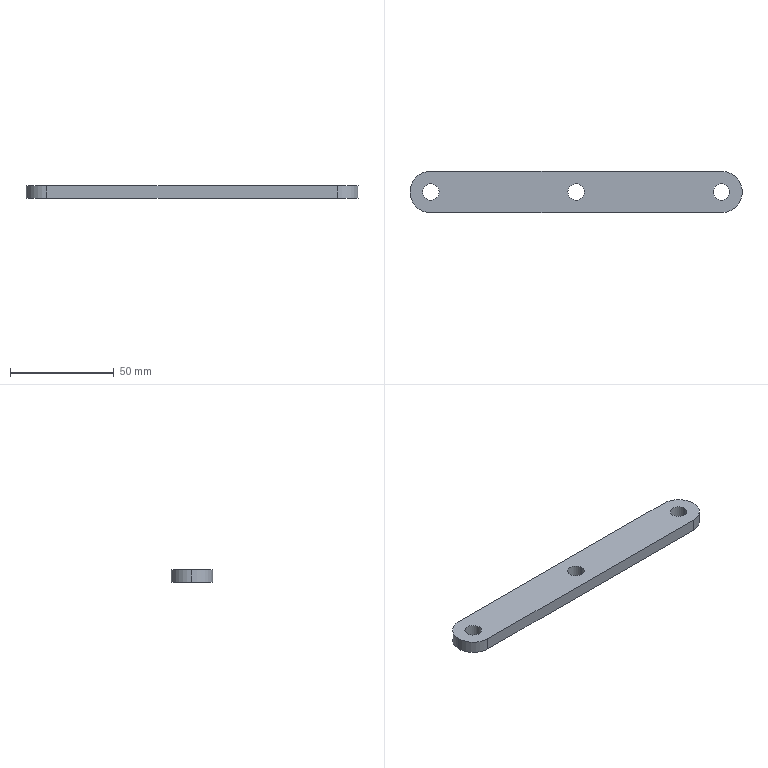Part | SolidWorks | features ICE 2, Extrusion 1 | 1 solid | 13 faces | box 160 x 20 x 6 mm | volume 17780 mm3 | cylinder 9 | plane 4 | commonest cylinder face diameters 8 x6 20 x3
STEP:
#1=CARTESIAN_POINT('',(66.,0.,0.));
#2=VERTEX_POINT('',#1);
#3=CARTESIAN_POINT('',(74.,0.,0.));
#4=VERTEX_POINT('',#3);
#5=CARTESIAN_POINT('',(70.,0.,0.));
#6=DIRECTION('',(0.,0.,1.));
#7=DIRECTION('',(1.,0.,0.));
#8=AXIS2_PLACEMENT_3D('',#5,#6,#7);
#9=CIRCLE('',#8,4.);
#10=EDGE_CURVE('',#2,#4,#9,.T.);
#11=ORIENTED_EDGE('',*,*,#10,.F.);
#12=CARTESIAN_POINT('',(66.,0.,6.));
#13=VERTEX_POINT('',#12);
#14=CARTESIAN_POINT('',(66.,0.,-4.));
#15=DIRECTION('',(0.,0.,1.));
#16=VECTOR('',#15,1000.);
#17=LINE('',#14,#16);
#18=EDGE_CURVE('',#2,#13,#17,.T.);
#19=ORIENTED_EDGE('',*,*,#18,.T.);
#20=CARTESIAN_POINT('',(74.,0.,6.));
#21=VERTEX_POINT('',#20);
#22=CARTESIAN_POINT('',(70.,0.,6.));
#23=DIRECTION('',(0.,0.,1.));
#24=DIRECTION('',(1.,0.,0.));
#25=AXIS2_PLACEMENT_3D('',#22,#23,#24);
#26=CIRCLE('',#25,4.);
#27=EDGE_CURVE('',#13,#21,#26,.T.);
#28=ORIENTED_EDGE('',*,*,#27,.T.);
#29=CARTESIAN_POINT('',(74.,0.,-4.));
#30=DIRECTION('',(0.,0.,1.));
#31=VECTOR('',#30,1000.);
#32=LINE('',#29,#31);
#33=EDGE_CURVE('',#4,#21,#32,.T.);
#34=ORIENTED_EDGE('',*,*,#33,.F.);
#35=EDGE_LOOP('',(#11,#19,#28,#34));
#36=FACE_OUTER_BOUND('',#35,.T.);
#37=CARTESIAN_POINT('',(70.,0.,-4.));
#38=DIRECTION('',(0.,0.,1.));
#39=DIRECTION('',(1.,0.,0.));
#40=AXIS2_PLACEMENT_3D('',#37,#38,#39);
#41=CYLINDRICAL_SURFACE('',#40,4.);
#42=ADVANCED_FACE('',(#36),#41,.F.);
#43=CARTESIAN_POINT('',(136.,0.,0.));
#44=VERTEX_POINT('',#43);
#45=CARTESIAN_POINT('',(144.,0.,0.));
#46=VERTEX_POINT('',#45);
#47=CARTESIAN_POINT('',(140.,0.,0.));
#48=DIRECTION('',(0.,0.,1.));
#49=DIRECTION('',(1.,0.,0.));
#50=AXIS2_PLACEMENT_3D('',#47,#48,#49);
#51=CIRCLE('',#50,4.);
#52=EDGE_CURVE('',#44,#46,#51,.T.);
#53=ORIENTED_EDGE('',*,*,#52,.F.);
#54=CARTESIAN_POINT('',(136.,0.,6.));
#55=VERTEX_POINT('',#54);
#56=CARTESIAN_POINT('',(136.,0.,-89.));
#57=DIRECTION('',(0.,0.,1.));
#58=VECTOR('',#57,1000.);
#59=LINE('',#56,#58);
#60=EDGE_CURVE('',#44,#55,#59,.T.);
#61=ORIENTED_EDGE('',*,*,#60,.T.);
#62=CARTESIAN_POINT('',(144.,0.,6.));
#63=VERTEX_POINT('',#62);
#64=CARTESIAN_POINT('',(140.,0.,6.));
#65=DIRECTION('',(0.,0.,1.));
#66=DIRECTION('',(1.,0.,0.));
#67=AXIS2_PLACEMENT_3D('',#64,#65,#66);
#68=CIRCLE('',#67,4.);
#69=EDGE_CURVE('',#55,#63,#68,.T.);
#70=ORIENTED_EDGE('',*,*,#69,.T.);
#71=CARTESIAN_POINT('',(144.,0.,-89.));
#72=DIRECTION('',(0.,0.,1.));
#73=VECTOR('',#72,1000.);
#74=LINE('',#71,#73);
#75=EDGE_CURVE('',#46,#63,#74,.T.);
#76=ORIENTED_EDGE('',*,*,#75,.F.);
#77=EDGE_LOOP('',(#53,#61,#70,#76));
#78=FACE_OUTER_BOUND('',#77,.T.);
#79=CARTESIAN_POINT('',(140.,0.,-89.));
#80=DIRECTION('',(0.,0.,1.));
#81=DIRECTION('',(1.,0.,0.));
#82=AXIS2_PLACEMENT_3D('',#79,#80,#81);
#83=CYLINDRICAL_SURFACE('',#82,4.);
#84=ADVANCED_FACE('',(#78),#83,.F.);
#85=CARTESIAN_POINT('',(-4.,0.,0.));
#86=VERTEX_POINT('',#85);
#87=CARTESIAN_POINT('',(4.,0.,0.));
#88=VERTEX_POINT('',#87);
#89=CARTESIAN_POINT('',(0.,0.,0.));
#90=DIRECTION('',(0.,0.,1.));
#91=DIRECTION('',(1.,0.,0.));
#92=AXIS2_PLACEMENT_3D('',#89,#90,#91);
#93=CIRCLE('',#92,4.);
#94=EDGE_CURVE('',#86,#88,#93,.T.);
#95=ORIENTED_EDGE('',*,*,#94,.F.);
#96=CARTESIAN_POINT('',(-4.,0.,6.));
#97=VERTEX_POINT('',#96);
#98=CARTESIAN_POINT('',(-4.,0.,-89.));
#99=DIRECTION('',(0.,0.,1.));
#100=VECTOR('',#99,1000.);
#101=LINE('',#98,#100);
#102=EDGE_CURVE('',#86,#97,#101,.T.);
#103=ORIENTED_EDGE('',*,*,#102,.T.);
#104=CARTESIAN_POINT('',(4.,0.,6.));
#105=VERTEX_POINT('',#104);
#106=CARTESIAN_POINT('',(0.,0.,6.));
#107=DIRECTION('',(0.,0.,1.));
#108=DIRECTION('',(1.,0.,0.));
#109=AXIS2_PLACEMENT_3D('',#106,#107,#108);
#110=CIRCLE('',#109,4.);
#111=EDGE_CURVE('',#97,#105,#110,.T.);
#112=ORIENTED_EDGE('',*,*,#111,.T.);
#113=CARTESIAN_POINT('',(4.,0.,-89.));
#114=DIRECTION('',(0.,0.,1.));
#115=VECTOR('',#114,1000.);
#116=LINE('',#113,#115);
#117=EDGE_CURVE('',#88,#105,#116,.T.);
#118=ORIENTED_EDGE('',*,*,#117,.F.);
#119=EDGE_LOOP('',(#95,#103,#112,#118));
#120=FACE_OUTER_BOUND('',#119,.T.);
#121=CARTESIAN_POINT('',(0.,0.,-89.));
#122=DIRECTION('',(0.,0.,1.));
#123=DIRECTION('',(1.,0.,0.));
#124=AXIS2_PLACEMENT_3D('',#121,#122,#123);
#125=CYLINDRICAL_SURFACE('',#124,4.);
#126=ADVANCED_FACE('',(#120),#125,.F.);
#127=CARTESIAN_POINT('',(-10.,0.,6.));
#128=VERTEX_POINT('',#127);
#129=CARTESIAN_POINT('',(0.,-10.,6.));
#130=VERTEX_POINT('',#129);
#131=CARTESIAN_POINT('',(0.,0.,6.));
#132=DIRECTION('',(0.,0.,1.));
#133=DIRECTION('',(1.,0.,0.));
#134=AXIS2_PLACEMENT_3D('',#131,#132,#133);
#135=CIRCLE('',#134,10.);
#136=EDGE_CURVE('',#128,#130,#135,.T.);
#137=ORIENTED_EDGE('',*,*,#136,.F.);
#138=CARTESIAN_POINT('',(-10.,0.,0.));
#139=VERTEX_POINT('',#138);
#140=CARTESIAN_POINT('',(-10.,0.,6.));
#141=DIRECTION('',(0.,0.,-1.));
#142=VECTOR('',#141,1000.);
#143=LINE('',#140,#142);
#144=EDGE_CURVE('',#128,#139,#143,.T.);
#145=ORIENTED_EDGE('',*,*,#144,.T.);
#146=CARTESIAN_POINT('',(0.,-10.,0.));
#147=VERTEX_POINT('',#146);
#148=CARTESIAN_POINT('',(0.,0.,0.));
#149=DIRECTION('',(0.,0.,1.));
#150=DIRECTION('',(1.,0.,0.));
#151=AXIS2_PLACEMENT_3D('',#148,#149,#150);
#152=CIRCLE('',#151,10.);
#153=EDGE_CURVE('',#139,#147,#152,.T.);
#154=ORIENTED_EDGE('',*,*,#153,.T.);
#155=CARTESIAN_POINT('',(0.,-10.,6.));
#156=DIRECTION('',(0.,0.,-1.));
#157=VECTOR('',#156,1000.);
#158=LINE('',#155,#157);
#159=EDGE_CURVE('',#130,#147,#158,.T.);
#160=ORIENTED_EDGE('',*,*,#159,.F.);
#161=EDGE_LOOP('',(#137,#145,#154,#160));
#162=FACE_OUTER_BOUND('',#161,.T.);
#163=CARTESIAN_POINT('',(0.,0.,6.));
#164=DIRECTION('',(0.,0.,-1.));
#165=DIRECTION('',(-1.,0.,0.));
#166=AXIS2_PLACEMENT_3D('',#163,#164,#165);
#167=CYLINDRICAL_SURFACE('',#166,10.);
#168=ADVANCED_FACE('',(#162),#167,.T.);
#169=ORIENTED_EDGE('',*,*,#144,.F.);
#170=CARTESIAN_POINT('',(0.,10.,6.));
#171=VERTEX_POINT('',#170);
#172=CARTESIAN_POINT('',(0.,0.,6.));
#173=DIRECTION('',(0.,0.,1.));
#174=DIRECTION('',(1.,0.,0.));
#175=AXIS2_PLACEMENT_3D('',#172,#173,#174);
#176=CIRCLE('',#175,10.);
#177=EDGE_CURVE('',#171,#128,#176,.T.);
#178=ORIENTED_EDGE('',*,*,#177,.F.);
#179=CARTESIAN_POINT('',(0.,10.,0.));
#180=VERTEX_POINT('',#179);
#181=CARTESIAN_POINT('',(0.,10.,6.));
#182=DIRECTION('',(0.,0.,-1.));
#183=VECTOR('',#182,1000.);
#184=LINE('',#181,#183);
#185=EDGE_CURVE('',#171,#180,#184,.T.);
#186=ORIENTED_EDGE('',*,*,#185,.T.);
#187=CARTESIAN_POINT('',(0.,0.,0.));
#188=DIRECTION('',(0.,0.,1.));
#189=DIRECTION('',(1.,0.,0.));
#190=AXIS2_PLACEMENT_3D('',#187,#188,#189);
#191=CIRCLE('',#190,10.);
#192=EDGE_CURVE('',#180,#139,#191,.T.);
#193=ORIENTED_EDGE('',*,*,#192,.T.);
#194=EDGE_LOOP('',(#169,#178,#186,#193));
#195=FACE_OUTER_BOUND('',#194,.T.);
#196=CARTESIAN_POINT('',(0.,0.,6.));
#197=DIRECTION('',(0.,0.,-1.));
#198=DIRECTION('',(-1.,0.,0.));
#199=AXIS2_PLACEMENT_3D('',#196,#197,#198);
#200=CYLINDRICAL_SURFACE('',#199,10.);
#201=ADVANCED_FACE('',(#195),#200,.T.);
#202=CARTESIAN_POINT('',(140.,-10.,0.));
#203=VERTEX_POINT('',#202);
#204=CARTESIAN_POINT('',(0.,-10.,0.));
#205=DIRECTION('',(1.,0.,0.));
#206=VECTOR('',#205,1000.);
#207=LINE('',#204,#206);
#208=EDGE_CURVE('',#147,#203,#207,.T.);
#209=ORIENTED_EDGE('',*,*,#208,.T.);
#210=CARTESIAN_POINT('',(140.,-10.,6.));
#211=VERTEX_POINT('',#210);
#212=CARTESIAN_POINT('',(140.,-10.,6.));
#213=DIRECTION('',(0.,0.,-1.));
#214=VECTOR('',#213,1000.);
#215=LINE('',#212,#214);
#216=EDGE_CURVE('',#211,#203,#215,.T.);
#217=ORIENTED_EDGE('',*,*,#216,.F.);
#218=CARTESIAN_POINT('',(0.,-10.,6.));
#219=DIRECTION('',(1.,0.,0.));
#220=VECTOR('',#219,1000.);
#221=LINE('',#218,#220);
#222=EDGE_CURVE('',#130,#211,#221,.T.);
#223=ORIENTED_EDGE('',*,*,#222,.F.);
#224=ORIENTED_EDGE('',*,*,#159,.T.);
#225=EDGE_LOOP('',(#209,#217,#223,#224));
#226=FACE_OUTER_BOUND('',#225,.T.);
#227=CARTESIAN_POINT('',(0.,-10.,6.));
#228=DIRECTION('',(0.,1.,0.));
#229=DIRECTION('',(-1.,0.,0.));
#230=AXIS2_PLACEMENT_3D('',#227,#228,#229);
#231=PLANE('',#230);
#232=ADVANCED_FACE('',(#226),#231,.F.);
#233=CARTESIAN_POINT('',(140.,10.,0.));
#234=VERTEX_POINT('',#233);
#235=CARTESIAN_POINT('',(140.,0.,0.));
#236=DIRECTION('',(0.,0.,1.));
#237=DIRECTION('',(1.,0.,0.));
#238=AXIS2_PLACEMENT_3D('',#235,#236,#237);
#239=CIRCLE('',#238,10.);
#240=EDGE_CURVE('',#203,#234,#239,.T.);
#241=ORIENTED_EDGE('',*,*,#240,.T.);
#242=CARTESIAN_POINT('',(140.,10.,6.));
#243=VERTEX_POINT('',#242);
#244=CARTESIAN_POINT('',(140.,10.,6.));
#245=DIRECTION('',(0.,0.,-1.));
#246=VECTOR('',#245,1000.);
#247=LINE('',#244,#246);
#248=EDGE_CURVE('',#243,#234,#247,.T.);
#249=ORIENTED_EDGE('',*,*,#248,.F.);
#250=CARTESIAN_POINT('',(140.,0.,6.));
#251=DIRECTION('',(0.,0.,1.));
#252=DIRECTION('',(1.,0.,0.));
#253=AXIS2_PLACEMENT_3D('',#250,#251,#252);
#254=CIRCLE('',#253,10.);
#255=EDGE_CURVE('',#211,#243,#254,.T.);
#256=ORIENTED_EDGE('',*,*,#255,.F.);
#257=ORIENTED_EDGE('',*,*,#216,.T.);
#258=EDGE_LOOP('',(#241,#249,#256,#257));
#259=FACE_OUTER_BOUND('',#258,.T.);
#260=CARTESIAN_POINT('',(140.,0.,6.));
#261=DIRECTION('',(0.,0.,-1.));
#262=DIRECTION('',(-1.,0.,0.));
#263=AXIS2_PLACEMENT_3D('',#260,#261,#262);
#264=CYLINDRICAL_SURFACE('',#263,10.);
#265=ADVANCED_FACE('',(#259),#264,.T.);
#266=CARTESIAN_POINT('',(0.,10.,0.));
#267=DIRECTION('',(-1.,0.,0.));
#268=VECTOR('',#267,1000.);
#269=LINE('',#266,#268);
#270=EDGE_CURVE('',#234,#180,#269,.T.);
#271=ORIENTED_EDGE('',*,*,#270,.T.);
#272=ORIENTED_EDGE('',*,*,#185,.F.);
#273=CARTESIAN_POINT('',(0.,10.,6.));
#274=DIRECTION('',(-1.,0.,0.));
#275=VECTOR('',#274,1000.);
#276=LINE('',#273,#275);
#277=EDGE_CURVE('',#243,#171,#276,.T.);
#278=ORIENTED_EDGE('',*,*,#277,.F.);
#279=ORIENTED_EDGE('',*,*,#248,.T.);
#280=EDGE_LOOP('',(#271,#272,#278,#279));
#281=FACE_OUTER_BOUND('',#280,.T.);
#282=CARTESIAN_POINT('',(0.,10.,6.));
#283=DIRECTION('',(0.,-1.,0.));
#284=DIRECTION('',(1.,0.,0.));
#285=AXIS2_PLACEMENT_3D('',#282,#283,#284);
#286=PLANE('',#285);
#287=ADVANCED_FACE('',(#281),#286,.F.);
#288=CARTESIAN_POINT('',(70.,0.,6.));
#289=DIRECTION('',(0.,0.,1.));
#290=DIRECTION('',(1.,0.,0.));
#291=AXIS2_PLACEMENT_3D('',#288,#289,#290);
#292=CIRCLE('',#291,4.);
#293=EDGE_CURVE('',#21,#13,#292,.T.);
#294=ORIENTED_EDGE('',*,*,#293,.F.);
#295=ORIENTED_EDGE('',*,*,#27,.F.);
#296=EDGE_LOOP('',(#294,#295));
#297=FACE_BOUND('',#296,.T.);
#298=CARTESIAN_POINT('',(140.,0.,6.));
#299=DIRECTION('',(0.,0.,1.));
#300=DIRECTION('',(1.,0.,0.));
#301=AXIS2_PLACEMENT_3D('',#298,#299,#300);
#302=CIRCLE('',#301,4.);
#303=EDGE_CURVE('',#63,#55,#302,.T.);
#304=ORIENTED_EDGE('',*,*,#303,.F.);
#305=ORIENTED_EDGE('',*,*,#69,.F.);
#306=EDGE_LOOP('',(#304,#305));
#307=FACE_BOUND('',#306,.T.);
#308=CARTESIAN_POINT('',(0.,0.,6.));
#309=DIRECTION('',(0.,0.,1.));
#310=DIRECTION('',(1.,0.,0.));
#311=AXIS2_PLACEMENT_3D('',#308,#309,#310);
#312=CIRCLE('',#311,4.);
#313=EDGE_CURVE('',#105,#97,#312,.T.);
#314=ORIENTED_EDGE('',*,*,#313,.F.);
#315=ORIENTED_EDGE('',*,*,#111,.F.);
#316=EDGE_LOOP('',(#314,#315));
#317=FACE_BOUND('',#316,.T.);
#318=ORIENTED_EDGE('',*,*,#177,.T.);
#319=ORIENTED_EDGE('',*,*,#136,.T.);
#320=ORIENTED_EDGE('',*,*,#222,.T.);
#321=ORIENTED_EDGE('',*,*,#255,.T.);
#322=ORIENTED_EDGE('',*,*,#277,.T.);
#323=EDGE_LOOP('',(#318,#319,#320,#321,#322));
#324=FACE_OUTER_BOUND('',#323,.T.);
#325=CARTESIAN_POINT('',(0.,0.,6.));
#326=DIRECTION('',(0.,0.,1.));
#327=DIRECTION('',(1.,0.,0.));
#328=AXIS2_PLACEMENT_3D('',#325,#326,#327);
#329=PLANE('',#328);
#330=ADVANCED_FACE('',(#297,#307,#317,#324),#329,.T.);
#331=CARTESIAN_POINT('',(70.,0.,0.));
#332=DIRECTION('',(0.,0.,1.));
#333=DIRECTION('',(1.,0.,0.));
#334=AXIS2_PLACEMENT_3D('',#331,#332,#333);
#335=CIRCLE('',#334,4.);
#336=EDGE_CURVE('',#4,#2,#335,.T.);
#337=ORIENTED_EDGE('',*,*,#336,.T.);
#338=ORIENTED_EDGE('',*,*,#10,.T.);
#339=EDGE_LOOP('',(#337,#338));
#340=FACE_BOUND('',#339,.T.);
#341=CARTESIAN_POINT('',(140.,0.,0.));
#342=DIRECTION('',(0.,0.,1.));
#343=DIRECTION('',(1.,0.,0.));
#344=AXIS2_PLACEMENT_3D('',#341,#342,#343);
#345=CIRCLE('',#344,4.);
#346=EDGE_CURVE('',#46,#44,#345,.T.);
#347=ORIENTED_EDGE('',*,*,#346,.T.);
#348=ORIENTED_EDGE('',*,*,#52,.T.);
#349=EDGE_LOOP('',(#347,#348));
#350=FACE_BOUND('',#349,.T.);
#351=CARTESIAN_POINT('',(0.,0.,0.));
#352=DIRECTION('',(0.,0.,1.));
#353=DIRECTION('',(1.,0.,0.));
#354=AXIS2_PLACEMENT_3D('',#351,#352,#353);
#355=CIRCLE('',#354,4.);
#356=EDGE_CURVE('',#88,#86,#355,.T.);
#357=ORIENTED_EDGE('',*,*,#356,.T.);
#358=ORIENTED_EDGE('',*,*,#94,.T.);
#359=EDGE_LOOP('',(#357,#358));
#360=FACE_BOUND('',#359,.T.);
#361=ORIENTED_EDGE('',*,*,#192,.F.);
#362=ORIENTED_EDGE('',*,*,#270,.F.);
#363=ORIENTED_EDGE('',*,*,#240,.F.);
#364=ORIENTED_EDGE('',*,*,#208,.F.);
#365=ORIENTED_EDGE('',*,*,#153,.F.);
#366=EDGE_LOOP('',(#361,#362,#363,#364,#365));
#367=FACE_OUTER_BOUND('',#366,.T.);
#368=CARTESIAN_POINT('',(0.,0.,0.));
#369=DIRECTION('',(0.,0.,1.));
#370=DIRECTION('',(1.,0.,0.));
#371=AXIS2_PLACEMENT_3D('',#368,#369,#370);
#372=PLANE('',#371);
#373=ADVANCED_FACE('',(#340,#350,#360,#367),#372,.F.);
#374=ORIENTED_EDGE('',*,*,#102,.F.);
#375=ORIENTED_EDGE('',*,*,#356,.F.);
#376=ORIENTED_EDGE('',*,*,#117,.T.);
#377=ORIENTED_EDGE('',*,*,#313,.T.);
#378=EDGE_LOOP('',(#374,#375,#376,#377));
#379=FACE_OUTER_BOUND('',#378,.T.);
#380=CARTESIAN_POINT('',(0.,0.,-89.));
#381=DIRECTION('',(0.,0.,1.));
#382=DIRECTION('',(1.,0.,0.));
#383=AXIS2_PLACEMENT_3D('',#380,#381,#382);
#384=CYLINDRICAL_SURFACE('',#383,4.);
#385=ADVANCED_FACE('',(#379),#384,.F.);
#386=ORIENTED_EDGE('',*,*,#60,.F.);
#387=ORIENTED_EDGE('',*,*,#346,.F.);
#388=ORIENTED_EDGE('',*,*,#75,.T.);
#389=ORIENTED_EDGE('',*,*,#303,.T.);
#390=EDGE_LOOP('',(#386,#387,#388,#389));
#391=FACE_OUTER_BOUND('',#390,.T.);
#392=CARTESIAN_POINT('',(140.,0.,-89.));
#393=DIRECTION('',(0.,0.,1.));
#394=DIRECTION('',(1.,0.,0.));
#395=AXIS2_PLACEMENT_3D('',#392,#393,#394);
#396=CYLINDRICAL_SURFACE('',#395,4.);
#397=ADVANCED_FACE('',(#391),#396,.F.);
#398=ORIENTED_EDGE('',*,*,#18,.F.);
#399=ORIENTED_EDGE('',*,*,#336,.F.);
#400=ORIENTED_EDGE('',*,*,#33,.T.);
#401=ORIENTED_EDGE('',*,*,#293,.T.);
#402=EDGE_LOOP('',(#398,#399,#400,#401));
#403=FACE_OUTER_BOUND('',#402,.T.);
#404=CARTESIAN_POINT('',(70.,0.,-4.));
#405=DIRECTION('',(0.,0.,1.));
#406=DIRECTION('',(1.,0.,0.));
#407=AXIS2_PLACEMENT_3D('',#404,#405,#406);
#408=CYLINDRICAL_SURFACE('',#407,4.);
#409=ADVANCED_FACE('',(#403),#408,.F.);
#410=CLOSED_SHELL('',(#42,#84,#126,#168,#201,#232,#265,#287,#330,#373,#385,#397,#409));
#411=MANIFOLD_SOLID_BREP('',#410);
#412=CARTESIAN_POINT('',(0.,0.,0.));
#413=DIRECTION('',(0.,0.,1.));
#414=DIRECTION('',(1.,0.,0.));
#415=AXIS2_PLACEMENT_3D('',#412,#413,#414);
#416=(LENGTH_UNIT()NAMED_UNIT(*)SI_UNIT(.MILLI.,.METRE.));
#417=UNCERTAINTY_MEASURE_WITH_UNIT(LENGTH_MEASURE(0.00001),#416,'','');
#418=(NAMED_UNIT(*)PLANE_ANGLE_UNIT()SI_UNIT($,.RADIAN.));
#419=(NAMED_UNIT(*)SI_UNIT($,.STERADIAN.)SOLID_ANGLE_UNIT());
#420=(GEOMETRIC_REPRESENTATION_CONTEXT(3)GLOBAL_UNCERTAINTY_ASSIGNED_CONTEXT((#417))GLOBAL_UNIT_ASSIGNED_CONTEXT((#416,#418,#419))REPRESENTATION_CONTEXT('',''));
#421=ADVANCED_BREP_SHAPE_REPRESENTATION('',(#411,#415),#420);